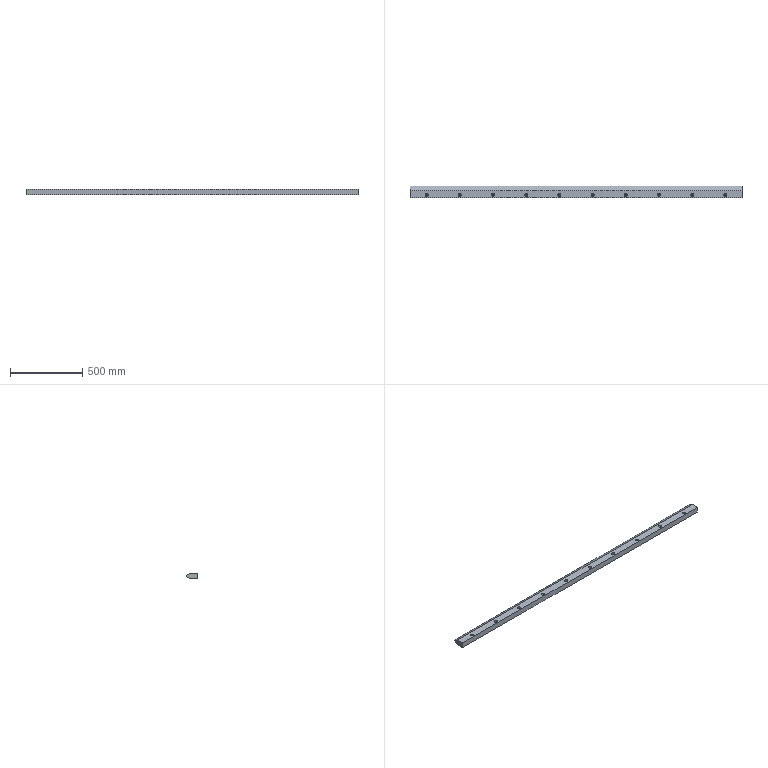Part | SolidWorks | features ICE 2, Extrusion 1, LPattern 1 | 1 solid | 58 faces | box 2300 x 80 x 40 mm | volume 6073150 mm3 | cylinder 40 | plane 18 | commonest cylinder face diameters 10 x20 22 x20